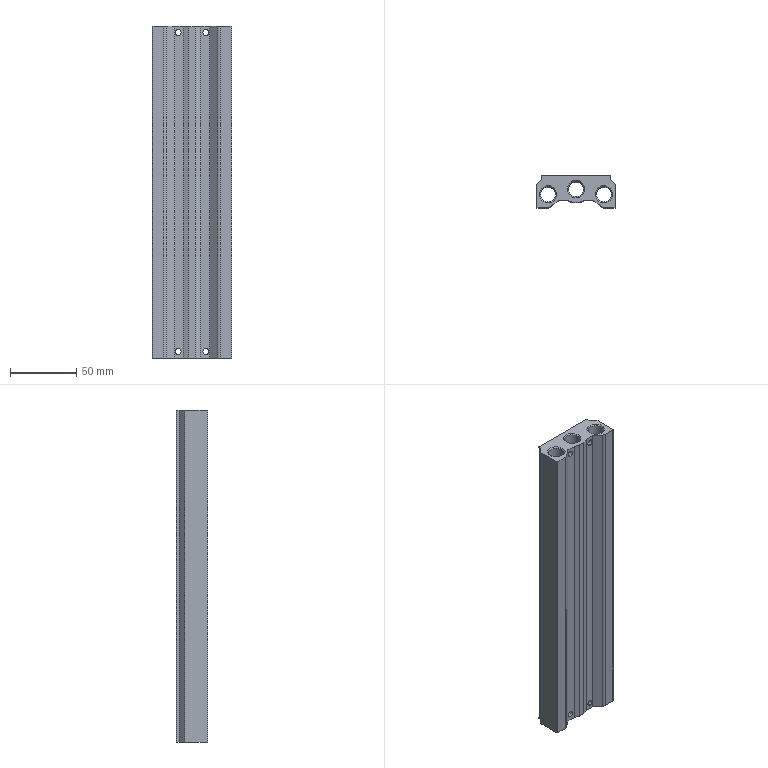Part | STEP file | 200M10F | 1 solid | 258 faces | box 60 x 24 x 251 mm | volume 220030 mm3 | cylinder 128 | cone 92 | plane 38 | commonest cylinder face diameters 2.459 x40 6.5 x40 10.2 x20 1 x12 4.5 x8 11.445 x6